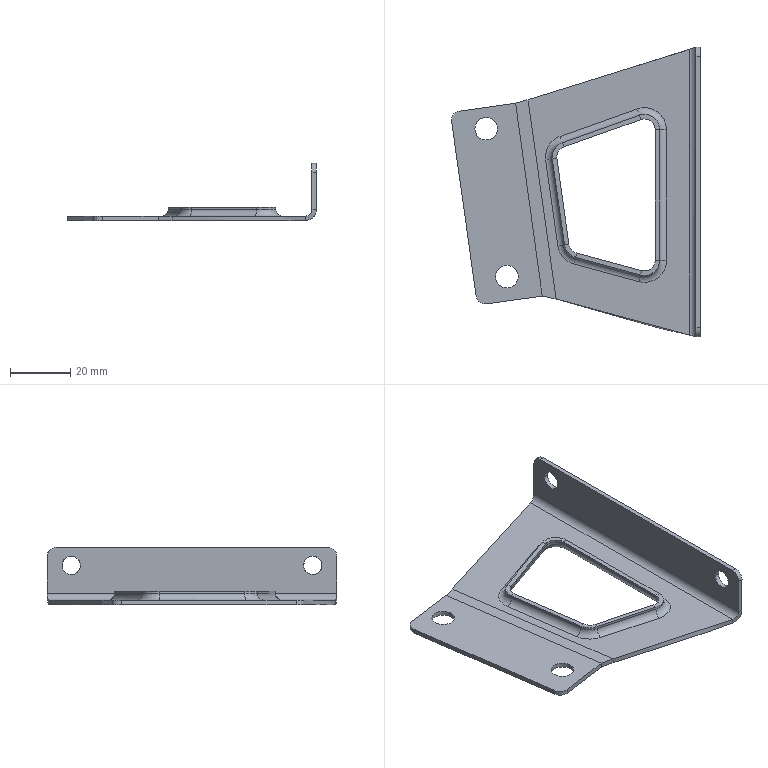Part | STEP file | gslz 2016.10.28-6_id38_x_t | 1 solid | 75 faces | box 82.449 x 96 x 19.004 mm | volume 9470 mm3 | plane 30 | cylinder 24 | spline 8 | torus 8 | other 5 | commonest cylinder face diameters 7.5 x7 4.5 x5 6 x4 7 x4 10 x4